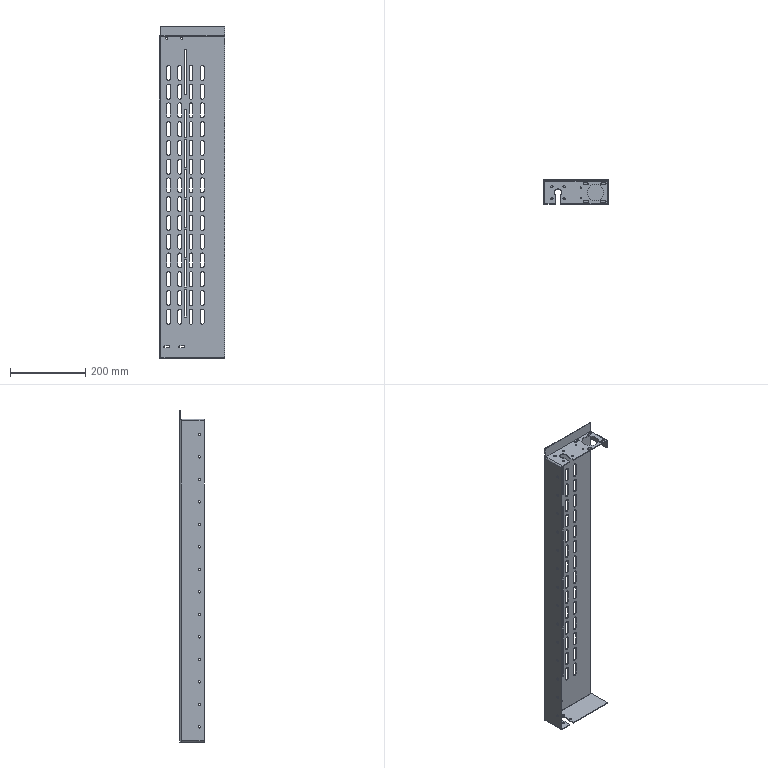Part | STEP file | Lead screw mechanism sheet metal V1.201001 | 1 solid | 455 faces | box 175 x 65 x 885 mm | volume 405761 mm3 | cylinder 276 | plane 179 | commonest cylinder face diameters 10 x168 6 x40 3.5 x28 5.5 x24 20 x6 4 x4